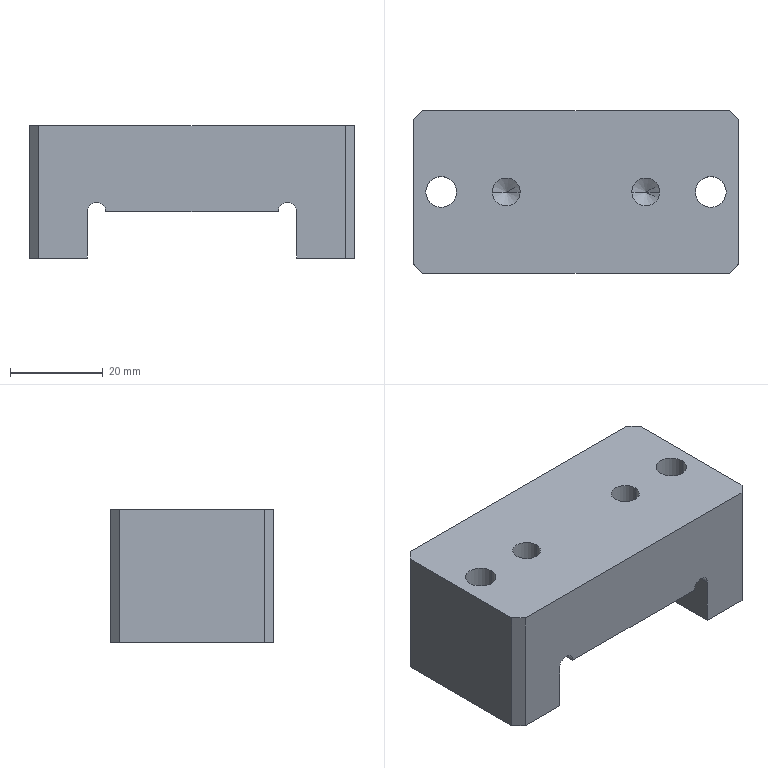Part | SolidWorks | features HoleWzd 3, Chamfer 1, Extrusion 1, ICE 1 | 1 solid | 52 faces | box 70 x 35 x 28.4 mm | volume 48866 mm3 | cylinder 24 | plane 16 | cone 12 | commonest cylinder face diameters 3.3 x8 4 x4 6 x4 6.6 x4 11 x4
STEP:
#1=CARTESIAN_POINT('',(30.65,12.5,-9.9));
#2=VERTEX_POINT('',#1);
#3=CARTESIAN_POINT('',(27.35,12.5,-9.9));
#4=VERTEX_POINT('',#3);
#5=CARTESIAN_POINT('',(29.,12.5,-9.9));
#6=DIRECTION('',(0.,0.,-1.));
#7=DIRECTION('',(-1.,0.,0.));
#8=AXIS2_PLACEMENT_3D('',#5,#6,#7);
#9=CIRCLE('',#8,1.65);
#10=EDGE_CURVE('',#2,#4,#9,.T.);
#11=ORIENTED_EDGE('',*,*,#10,.F.);
#12=CARTESIAN_POINT('',(30.65,12.5,-28.4));
#13=VERTEX_POINT('',#12);
#14=CARTESIAN_POINT('',(30.65,12.5,-28.4));
#15=DIRECTION('',(0.,0.,-1.));
#16=VECTOR('',#15,1000.);
#17=LINE('',#14,#16);
#18=EDGE_CURVE('',#2,#13,#17,.T.);
#19=ORIENTED_EDGE('',*,*,#18,.T.);
#20=CARTESIAN_POINT('',(27.35,12.5,-28.4));
#21=VERTEX_POINT('',#20);
#22=CARTESIAN_POINT('',(29.,12.5,-28.4));
#23=DIRECTION('',(0.,0.,-1.));
#24=DIRECTION('',(-1.,0.,0.));
#25=AXIS2_PLACEMENT_3D('',#22,#23,#24);
#26=CIRCLE('',#25,1.65);
#27=EDGE_CURVE('',#13,#21,#26,.T.);
#28=ORIENTED_EDGE('',*,*,#27,.T.);
#29=CARTESIAN_POINT('',(27.35,12.5,-28.4));
#30=DIRECTION('',(0.,0.,-1.));
#31=VECTOR('',#30,1000.);
#32=LINE('',#29,#31);
#33=EDGE_CURVE('',#4,#21,#32,.T.);
#34=ORIENTED_EDGE('',*,*,#33,.F.);
#35=EDGE_LOOP('',(#11,#19,#28,#34));
#36=FACE_OUTER_BOUND('',#35,.T.);
#37=CARTESIAN_POINT('',(29.,12.5,-28.4));
#38=DIRECTION('',(0.,0.,-1.));
#39=DIRECTION('',(-1.,0.,0.));
#40=AXIS2_PLACEMENT_3D('',#37,#38,#39);
#41=CYLINDRICAL_SURFACE('',#40,1.65);
#42=ADVANCED_FACE('',(#36),#41,.F.);
#43=CARTESIAN_POINT('',(29.,12.5,-8.909));
#44=VERTEX_POINT('',#43);
#45=CARTESIAN_POINT('',(27.35,12.5,-9.9));
#46=DIRECTION('',(-0.8572,0.,-0.515));
#47=VECTOR('',#46,1000.);
#48=LINE('',#45,#47);
#49=EDGE_CURVE('',#44,#4,#48,.T.);
#50=ORIENTED_EDGE('',*,*,#49,.F.);
#51=CARTESIAN_POINT('',(30.65,12.5,-9.9));
#52=DIRECTION('',(0.8572,0.,-0.515));
#53=VECTOR('',#52,1000.);
#54=LINE('',#51,#53);
#55=EDGE_CURVE('',#44,#2,#54,.T.);
#56=ORIENTED_EDGE('',*,*,#55,.T.);
#57=ORIENTED_EDGE('',*,*,#10,.T.);
#58=EDGE_LOOP('',(#50,#56,#57));
#59=FACE_OUTER_BOUND('',#58,.T.);
#60=CARTESIAN_POINT('',(29.,12.5,-9.9));
#61=DIRECTION('',(0.,0.,-1.));
#62=DIRECTION('',(-1.,0.,0.));
#63=AXIS2_PLACEMENT_3D('',#60,#61,#62);
#64=CONICAL_SURFACE('',#63,1.65,1.03);
#65=ADVANCED_FACE('',(#59),#64,.F.);
#66=CARTESIAN_POINT('',(30.65,-12.5,-9.9));
#67=VERTEX_POINT('',#66);
#68=CARTESIAN_POINT('',(27.35,-12.5,-9.9));
#69=VERTEX_POINT('',#68);
#70=CARTESIAN_POINT('',(29.,-12.5,-9.9));
#71=DIRECTION('',(0.,0.,-1.));
#72=DIRECTION('',(-1.,0.,0.));
#73=AXIS2_PLACEMENT_3D('',#70,#71,#72);
#74=CIRCLE('',#73,1.65);
#75=EDGE_CURVE('',#67,#69,#74,.T.);
#76=ORIENTED_EDGE('',*,*,#75,.F.);
#77=CARTESIAN_POINT('',(30.65,-12.5,-28.4));
#78=VERTEX_POINT('',#77);
#79=CARTESIAN_POINT('',(30.65,-12.5,-28.4));
#80=DIRECTION('',(0.,0.,-1.));
#81=VECTOR('',#80,1000.);
#82=LINE('',#79,#81);
#83=EDGE_CURVE('',#67,#78,#82,.T.);
#84=ORIENTED_EDGE('',*,*,#83,.T.);
#85=CARTESIAN_POINT('',(27.35,-12.5,-28.4));
#86=VERTEX_POINT('',#85);
#87=CARTESIAN_POINT('',(29.,-12.5,-28.4));
#88=DIRECTION('',(0.,0.,-1.));
#89=DIRECTION('',(-1.,0.,0.));
#90=AXIS2_PLACEMENT_3D('',#87,#88,#89);
#91=CIRCLE('',#90,1.65);
#92=EDGE_CURVE('',#78,#86,#91,.T.);
#93=ORIENTED_EDGE('',*,*,#92,.T.);
#94=CARTESIAN_POINT('',(27.35,-12.5,-28.4));
#95=DIRECTION('',(0.,0.,-1.));
#96=VECTOR('',#95,1000.);
#97=LINE('',#94,#96);
#98=EDGE_CURVE('',#69,#86,#97,.T.);
#99=ORIENTED_EDGE('',*,*,#98,.F.);
#100=EDGE_LOOP('',(#76,#84,#93,#99));
#101=FACE_OUTER_BOUND('',#100,.T.);
#102=CARTESIAN_POINT('',(29.,-12.5,-28.4));
#103=DIRECTION('',(0.,0.,-1.));
#104=DIRECTION('',(-1.,0.,0.));
#105=AXIS2_PLACEMENT_3D('',#102,#103,#104);
#106=CYLINDRICAL_SURFACE('',#105,1.65);
#107=ADVANCED_FACE('',(#101),#106,.F.);
#108=CARTESIAN_POINT('',(29.,-12.5,-8.909));
#109=VERTEX_POINT('',#108);
#110=CARTESIAN_POINT('',(27.35,-12.5,-9.9));
#111=DIRECTION('',(-0.8572,0.,-0.515));
#112=VECTOR('',#111,1000.);
#113=LINE('',#110,#112);
#114=EDGE_CURVE('',#109,#69,#113,.T.);
#115=ORIENTED_EDGE('',*,*,#114,.F.);
#116=CARTESIAN_POINT('',(30.65,-12.5,-9.9));
#117=DIRECTION('',(0.8572,0.,-0.515));
#118=VECTOR('',#117,1000.);
#119=LINE('',#116,#118);
#120=EDGE_CURVE('',#109,#67,#119,.T.);
#121=ORIENTED_EDGE('',*,*,#120,.T.);
#122=ORIENTED_EDGE('',*,*,#75,.T.);
#123=EDGE_LOOP('',(#115,#121,#122));
#124=FACE_OUTER_BOUND('',#123,.T.);
#125=CARTESIAN_POINT('',(29.,-12.5,-9.9));
#126=DIRECTION('',(0.,0.,-1.));
#127=DIRECTION('',(-1.,0.,0.));
#128=AXIS2_PLACEMENT_3D('',#125,#126,#127);
#129=CONICAL_SURFACE('',#128,1.65,1.03);
#130=ADVANCED_FACE('',(#124),#129,.F.);
#131=CARTESIAN_POINT('',(-27.35,12.5,-9.9));
#132=VERTEX_POINT('',#131);
#133=CARTESIAN_POINT('',(-30.65,12.5,-9.9));
#134=VERTEX_POINT('',#133);
#135=CARTESIAN_POINT('',(-29.,12.5,-9.9));
#136=DIRECTION('',(0.,0.,-1.));
#137=DIRECTION('',(-1.,0.,0.));
#138=AXIS2_PLACEMENT_3D('',#135,#136,#137);
#139=CIRCLE('',#138,1.65);
#140=EDGE_CURVE('',#132,#134,#139,.T.);
#141=ORIENTED_EDGE('',*,*,#140,.F.);
#142=CARTESIAN_POINT('',(-27.35,12.5,-28.4));
#143=VERTEX_POINT('',#142);
#144=CARTESIAN_POINT('',(-27.35,12.5,-28.4));
#145=DIRECTION('',(0.,0.,-1.));
#146=VECTOR('',#145,1000.);
#147=LINE('',#144,#146);
#148=EDGE_CURVE('',#132,#143,#147,.T.);
#149=ORIENTED_EDGE('',*,*,#148,.T.);
#150=CARTESIAN_POINT('',(-30.65,12.5,-28.4));
#151=VERTEX_POINT('',#150);
#152=CARTESIAN_POINT('',(-29.,12.5,-28.4));
#153=DIRECTION('',(0.,0.,-1.));
#154=DIRECTION('',(-1.,0.,0.));
#155=AXIS2_PLACEMENT_3D('',#152,#153,#154);
#156=CIRCLE('',#155,1.65);
#157=EDGE_CURVE('',#143,#151,#156,.T.);
#158=ORIENTED_EDGE('',*,*,#157,.T.);
#159=CARTESIAN_POINT('',(-30.65,12.5,-28.4));
#160=DIRECTION('',(0.,0.,-1.));
#161=VECTOR('',#160,1000.);
#162=LINE('',#159,#161);
#163=EDGE_CURVE('',#134,#151,#162,.T.);
#164=ORIENTED_EDGE('',*,*,#163,.F.);
#165=EDGE_LOOP('',(#141,#149,#158,#164));
#166=FACE_OUTER_BOUND('',#165,.T.);
#167=CARTESIAN_POINT('',(-29.,12.5,-28.4));
#168=DIRECTION('',(0.,0.,-1.));
#169=DIRECTION('',(-1.,0.,0.));
#170=AXIS2_PLACEMENT_3D('',#167,#168,#169);
#171=CYLINDRICAL_SURFACE('',#170,1.65);
#172=ADVANCED_FACE('',(#166),#171,.F.);
#173=CARTESIAN_POINT('',(-29.,12.5,-8.909));
#174=VERTEX_POINT('',#173);
#175=CARTESIAN_POINT('',(-30.65,12.5,-9.9));
#176=DIRECTION('',(-0.8572,0.,-0.515));
#177=VECTOR('',#176,1000.);
#178=LINE('',#175,#177);
#179=EDGE_CURVE('',#174,#134,#178,.T.);
#180=ORIENTED_EDGE('',*,*,#179,.F.);
#181=CARTESIAN_POINT('',(-27.35,12.5,-9.9));
#182=DIRECTION('',(0.8572,0.,-0.515));
#183=VECTOR('',#182,1000.);
#184=LINE('',#181,#183);
#185=EDGE_CURVE('',#174,#132,#184,.T.);
#186=ORIENTED_EDGE('',*,*,#185,.T.);
#187=ORIENTED_EDGE('',*,*,#140,.T.);
#188=EDGE_LOOP('',(#180,#186,#187));
#189=FACE_OUTER_BOUND('',#188,.T.);
#190=CARTESIAN_POINT('',(-29.,12.5,-9.9));
#191=DIRECTION('',(0.,0.,-1.));
#192=DIRECTION('',(-1.,0.,0.));
#193=AXIS2_PLACEMENT_3D('',#190,#191,#192);
#194=CONICAL_SURFACE('',#193,1.65,1.03);
#195=ADVANCED_FACE('',(#189),#194,.F.);
#196=CARTESIAN_POINT('',(-27.35,-12.5,-9.9));
#197=VERTEX_POINT('',#196);
#198=CARTESIAN_POINT('',(-30.65,-12.5,-9.9));
#199=VERTEX_POINT('',#198);
#200=CARTESIAN_POINT('',(-29.,-12.5,-9.9));
#201=DIRECTION('',(0.,0.,-1.));
#202=DIRECTION('',(-1.,0.,0.));
#203=AXIS2_PLACEMENT_3D('',#200,#201,#202);
#204=CIRCLE('',#203,1.65);
#205=EDGE_CURVE('',#197,#199,#204,.T.);
#206=ORIENTED_EDGE('',*,*,#205,.F.);
#207=CARTESIAN_POINT('',(-27.35,-12.5,-28.4));
#208=VERTEX_POINT('',#207);
#209=CARTESIAN_POINT('',(-27.35,-12.5,-28.4));
#210=DIRECTION('',(0.,0.,-1.));
#211=VECTOR('',#210,1000.);
#212=LINE('',#209,#211);
#213=EDGE_CURVE('',#197,#208,#212,.T.);
#214=ORIENTED_EDGE('',*,*,#213,.T.);
#215=CARTESIAN_POINT('',(-30.65,-12.5,-28.4));
#216=VERTEX_POINT('',#215);
#217=CARTESIAN_POINT('',(-29.,-12.5,-28.4));
#218=DIRECTION('',(0.,0.,-1.));
#219=DIRECTION('',(-1.,0.,0.));
#220=AXIS2_PLACEMENT_3D('',#217,#218,#219);
#221=CIRCLE('',#220,1.65);
#222=EDGE_CURVE('',#208,#216,#221,.T.);
#223=ORIENTED_EDGE('',*,*,#222,.T.);
#224=CARTESIAN_POINT('',(-30.65,-12.5,-28.4));
#225=DIRECTION('',(0.,0.,-1.));
#226=VECTOR('',#225,1000.);
#227=LINE('',#224,#226);
#228=EDGE_CURVE('',#199,#216,#227,.T.);
#229=ORIENTED_EDGE('',*,*,#228,.F.);
#230=EDGE_LOOP('',(#206,#214,#223,#229));
#231=FACE_OUTER_BOUND('',#230,.T.);
#232=CARTESIAN_POINT('',(-29.,-12.5,-28.4));
#233=DIRECTION('',(0.,0.,-1.));
#234=DIRECTION('',(-1.,0.,0.));
#235=AXIS2_PLACEMENT_3D('',#232,#233,#234);
#236=CYLINDRICAL_SURFACE('',#235,1.65);
#237=ADVANCED_FACE('',(#231),#236,.F.);
#238=CARTESIAN_POINT('',(-29.,-12.5,-8.909));
#239=VERTEX_POINT('',#238);
#240=CARTESIAN_POINT('',(-30.65,-12.5,-9.9));
#241=DIRECTION('',(-0.8572,0.,-0.515));
#242=VECTOR('',#241,1000.);
#243=LINE('',#240,#242);
#244=EDGE_CURVE('',#239,#199,#243,.T.);
#245=ORIENTED_EDGE('',*,*,#244,.F.);
#246=CARTESIAN_POINT('',(-27.35,-12.5,-9.9));
#247=DIRECTION('',(0.8572,0.,-0.515));
#248=VECTOR('',#247,1000.);
#249=LINE('',#246,#248);
#250=EDGE_CURVE('',#239,#197,#249,.T.);
#251=ORIENTED_EDGE('',*,*,#250,.T.);
#252=ORIENTED_EDGE('',*,*,#205,.T.);
#253=EDGE_LOOP('',(#245,#251,#252));
#254=FACE_OUTER_BOUND('',#253,.T.);
#255=CARTESIAN_POINT('',(-29.,-12.5,-9.9));
#256=DIRECTION('',(0.,0.,-1.));
#257=DIRECTION('',(-1.,0.,0.));
#258=AXIS2_PLACEMENT_3D('',#255,#256,#257);
#259=CONICAL_SURFACE('',#258,1.65,1.03);
#260=ADVANCED_FACE('',(#254),#259,.F.);
#261=CARTESIAN_POINT('',(34.5,0.,-21.6));
#262=VERTEX_POINT('',#261);
#263=CARTESIAN_POINT('',(23.5,0.,-21.6));
#264=VERTEX_POINT('',#263);
#265=CARTESIAN_POINT('',(29.,0.,-21.6));
#266=DIRECTION('',(0.,0.,-1.));
#267=DIRECTION('',(-1.,0.,0.));
#268=AXIS2_PLACEMENT_3D('',#265,#266,#267);
#269=CIRCLE('',#268,5.5);
#270=EDGE_CURVE('',#262,#264,#269,.T.);
#271=ORIENTED_EDGE('',*,*,#270,.F.);
#272=CARTESIAN_POINT('',(34.5,0.,-28.4));
#273=VERTEX_POINT('',#272);
#274=CARTESIAN_POINT('',(34.5,0.,-28.4));
#275=DIRECTION('',(0.,0.,-1.));
#276=VECTOR('',#275,1000.);
#277=LINE('',#274,#276);
#278=EDGE_CURVE('',#262,#273,#277,.T.);
#279=ORIENTED_EDGE('',*,*,#278,.T.);
#280=CARTESIAN_POINT('',(23.5,0.,-28.4));
#281=VERTEX_POINT('',#280);
#282=CARTESIAN_POINT('',(29.,0.,-28.4));
#283=DIRECTION('',(0.,0.,-1.));
#284=DIRECTION('',(-1.,0.,0.));
#285=AXIS2_PLACEMENT_3D('',#282,#283,#284);
#286=CIRCLE('',#285,5.5);
#287=EDGE_CURVE('',#273,#281,#286,.T.);
#288=ORIENTED_EDGE('',*,*,#287,.T.);
#289=CARTESIAN_POINT('',(23.5,0.,-28.4));
#290=DIRECTION('',(0.,0.,-1.));
#291=VECTOR('',#290,1000.);
#292=LINE('',#289,#291);
#293=EDGE_CURVE('',#264,#281,#292,.T.);
#294=ORIENTED_EDGE('',*,*,#293,.F.);
#295=EDGE_LOOP('',(#271,#279,#288,#294));
#296=FACE_OUTER_BOUND('',#295,.T.);
#297=CARTESIAN_POINT('',(29.,0.,-28.4));
#298=DIRECTION('',(0.,0.,-1.));
#299=DIRECTION('',(-1.,0.,0.));
#300=AXIS2_PLACEMENT_3D('',#297,#298,#299);
#301=CYLINDRICAL_SURFACE('',#300,5.5);
#302=ADVANCED_FACE('',(#296),#301,.F.);
#303=CARTESIAN_POINT('',(32.3,0.,0.));
#304=VERTEX_POINT('',#303);
#305=CARTESIAN_POINT('',(25.7,0.,0.));
#306=VERTEX_POINT('',#305);
#307=CARTESIAN_POINT('',(29.,0.,0.));
#308=DIRECTION('',(0.,0.,-1.));
#309=DIRECTION('',(-1.,0.,0.));
#310=AXIS2_PLACEMENT_3D('',#307,#308,#309);
#311=CIRCLE('',#310,3.3);
#312=EDGE_CURVE('',#304,#306,#311,.T.);
#313=ORIENTED_EDGE('',*,*,#312,.F.);
#314=CARTESIAN_POINT('',(32.3,0.,-21.6));
#315=VERTEX_POINT('',#314);
#316=CARTESIAN_POINT('',(32.3,0.,-28.4));
#317=DIRECTION('',(0.,0.,-1.));
#318=VECTOR('',#317,1000.);
#319=LINE('',#316,#318);
#320=EDGE_CURVE('',#304,#315,#319,.T.);
#321=ORIENTED_EDGE('',*,*,#320,.T.);
#322=CARTESIAN_POINT('',(25.7,0.,-21.6));
#323=VERTEX_POINT('',#322);
#324=CARTESIAN_POINT('',(29.,0.,-21.6));
#325=DIRECTION('',(0.,0.,-1.));
#326=DIRECTION('',(-1.,0.,0.));
#327=AXIS2_PLACEMENT_3D('',#324,#325,#326);
#328=CIRCLE('',#327,3.3);
#329=EDGE_CURVE('',#315,#323,#328,.T.);
#330=ORIENTED_EDGE('',*,*,#329,.T.);
#331=CARTESIAN_POINT('',(25.7,0.,-28.4));
#332=DIRECTION('',(0.,0.,-1.));
#333=VECTOR('',#332,1000.);
#334=LINE('',#331,#333);
#335=EDGE_CURVE('',#306,#323,#334,.T.);
#336=ORIENTED_EDGE('',*,*,#335,.F.);
#337=EDGE_LOOP('',(#313,#321,#330,#336));
#338=FACE_OUTER_BOUND('',#337,.T.);
#339=CARTESIAN_POINT('',(29.,0.,-28.4));
#340=DIRECTION('',(0.,0.,-1.));
#341=DIRECTION('',(-1.,0.,0.));
#342=AXIS2_PLACEMENT_3D('',#339,#340,#341);
#343=CYLINDRICAL_SURFACE('',#342,3.3);
#344=ADVANCED_FACE('',(#338),#343,.F.);
#345=CARTESIAN_POINT('',(-23.5,0.,-21.6));
#346=VERTEX_POINT('',#345);
#347=CARTESIAN_POINT('',(-34.5,0.,-21.6));
#348=VERTEX_POINT('',#347);
#349=CARTESIAN_POINT('',(-29.,0.,-21.6));
#350=DIRECTION('',(0.,0.,-1.));
#351=DIRECTION('',(-1.,0.,0.));
#352=AXIS2_PLACEMENT_3D('',#349,#350,#351);
#353=CIRCLE('',#352,5.5);
#354=EDGE_CURVE('',#346,#348,#353,.T.);
#355=ORIENTED_EDGE('',*,*,#354,.F.);
#356=CARTESIAN_POINT('',(-23.5,0.,-28.4));
#357=VERTEX_POINT('',#356);
#358=CARTESIAN_POINT('',(-23.5,0.,-28.4));
#359=DIRECTION('',(0.,0.,-1.));
#360=VECTOR('',#359,1000.);
#361=LINE('',#358,#360);
#362=EDGE_CURVE('',#346,#357,#361,.T.);
#363=ORIENTED_EDGE('',*,*,#362,.T.);
#364=CARTESIAN_POINT('',(-34.5,0.,-28.4));
#365=VERTEX_POINT('',#364);
#366=CARTESIAN_POINT('',(-29.,0.,-28.4));
#367=DIRECTION('',(0.,0.,-1.));
#368=DIRECTION('',(-1.,0.,0.));
#369=AXIS2_PLACEMENT_3D('',#366,#367,#368);
#370=CIRCLE('',#369,5.5);
#371=EDGE_CURVE('',#357,#365,#370,.T.);
#372=ORIENTED_EDGE('',*,*,#371,.T.);
#373=CARTESIAN_POINT('',(-34.5,0.,-28.4));
#374=DIRECTION('',(0.,0.,-1.));
#375=VECTOR('',#374,1000.);
#376=LINE('',#373,#375);
#377=EDGE_CURVE('',#348,#365,#376,.T.);
#378=ORIENTED_EDGE('',*,*,#377,.F.);
#379=EDGE_LOOP('',(#355,#363,#372,#378));
#380=FACE_OUTER_BOUND('',#379,.T.);
#381=CARTESIAN_POINT('',(-29.,0.,-28.4));
#382=DIRECTION('',(0.,0.,-1.));
#383=DIRECTION('',(-1.,0.,0.));
#384=AXIS2_PLACEMENT_3D('',#381,#382,#383);
#385=CYLINDRICAL_SURFACE('',#384,5.5);
#386=ADVANCED_FACE('',(#380),#385,.F.);
#387=CARTESIAN_POINT('',(-25.7,0.,0.));
#388=VERTEX_POINT('',#387);
#389=CARTESIAN_POINT('',(-32.3,0.,0.));
#390=VERTEX_POINT('',#389);
#391=CARTESIAN_POINT('',(-29.,0.,0.));
#392=DIRECTION('',(0.,0.,-1.));
#393=DIRECTION('',(-1.,0.,0.));
#394=AXIS2_PLACEMENT_3D('',#391,#392,#393);
#395=CIRCLE('',#394,3.3);
#396=EDGE_CURVE('',#388,#390,#395,.T.);
#397=ORIENTED_EDGE('',*,*,#396,.F.);
#398=CARTESIAN_POINT('',(-25.7,0.,-21.6));
#399=VERTEX_POINT('',#398);
#400=CARTESIAN_POINT('',(-25.7,0.,-28.4));
#401=DIRECTION('',(0.,0.,-1.));
#402=VECTOR('',#401,1000.);
#403=LINE('',#400,#402);
#404=EDGE_CURVE('',#388,#399,#403,.T.);
#405=ORIENTED_EDGE('',*,*,#404,.T.);
#406=CARTESIAN_POINT('',(-32.3,0.,-21.6));
#407=VERTEX_POINT('',#406);
#408=CARTESIAN_POINT('',(-29.,0.,-21.6));
#409=DIRECTION('',(0.,0.,-1.));
#410=DIRECTION('',(-1.,0.,0.));
#411=AXIS2_PLACEMENT_3D('',#408,#409,#410);
#412=CIRCLE('',#411,3.3);
#413=EDGE_CURVE('',#399,#407,#412,.T.);
#414=ORIENTED_EDGE('',*,*,#413,.T.);
#415=CARTESIAN_POINT('',(-32.3,0.,-28.4));
#416=DIRECTION('',(0.,0.,-1.));
#417=VECTOR('',#416,1000.);
#418=LINE('',#415,#417);
#419=EDGE_CURVE('',#390,#407,#418,.T.);
#420=ORIENTED_EDGE('',*,*,#419,.F.);
#421=EDGE_LOOP('',(#397,#405,#414,#420));
#422=FACE_OUTER_BOUND('',#421,.T.);
#423=CARTESIAN_POINT('',(-29.,0.,-28.4));
#424=DIRECTION('',(0.,0.,-1.));
#425=DIRECTION('',(-1.,0.,0.));
#426=AXIS2_PLACEMENT_3D('',#423,#424,#425);
#427=CYLINDRICAL_SURFACE('',#426,3.3);
#428=ADVANCED_FACE('',(#422),#427,.F.);
#429=CARTESIAN_POINT('',(-18.,0.,-15.));
#430=VERTEX_POINT('',#429);
#431=CARTESIAN_POINT('',(-12.,0.,-15.));
#432=VERTEX_POINT('',#431);
#433=CARTESIAN_POINT('',(-15.,0.,-15.));
#434=DIRECTION('',(0.,0.,1.));
#435=DIRECTION('',(1.,0.,0.));
#436=AXIS2_PLACEMENT_3D('',#433,#434,#435);
#437=CIRCLE('',#436,3.);
#438=EDGE_CURVE('',#430,#432,#437,.T.);
#439=ORIENTED_EDGE('',*,*,#438,.F.);
#440=CARTESIAN_POINT('',(-18.,0.,0.));
#441=VERTEX_POINT('',#440);
#442=CARTESIAN_POINT('',(-18.,0.,0.));
#443=DIRECTION('',(0.,0.,1.));
#444=VECTOR('',#443,1000.);
#445=LINE('',#442,#444);
#446=EDGE_CURVE('',#430,#441,#445,.T.);
#447=ORIENTED_EDGE('',*,*,#446,.T.);
#448=CARTESIAN_POINT('',(-12.,0.,0.));
#449=VERTEX_POINT('',#448);
#450=CARTESIAN_POINT('',(-15.,0.,0.));
#451=DIRECTION('',(0.,0.,1.));
#452=DIRECTION('',(1.,0.,0.));
#453=AXIS2_PLACEMENT_3D('',#450,#451,#452);
#454=CIRCLE('',#453,3.);
#455=EDGE_CURVE('',#441,#449,#454,.T.);
#456=ORIENTED_EDGE('',*,*,#455,.T.);
#457=CARTESIAN_POINT('',(-12.,0.,0.));
#458=DIRECTION('',(0.,0.,1.));
#459=VECTOR('',#458,1000.);
#460=LINE('',#457,#459);
#461=EDGE_CURVE('',#432,#449,#460,.T.);
#462=ORIENTED_EDGE('',*,*,#461,.F.);
#463=EDGE_LOOP('',(#439,#447,#456,#462));
#464=FACE_OUTER_BOUND('',#463,.T.);
#465=CARTESIAN_POINT('',(-15.,0.,0.));
#466=DIRECTION('',(0.,0.,1.));
#467=DIRECTION('',(1.,0.,0.));
#468=AXIS2_PLACEMENT_3D('',#465,#466,#467);
#469=CYLINDRICAL_SURFACE('',#468,3.);
#470=ADVANCED_FACE('',(#464),#469,.F.);
#471=CARTESIAN_POINT('',(-15.,0.,-16.803));
#472=VERTEX_POINT('',#471);
#473=CARTESIAN_POINT('',(-12.,0.,-15.));
#474=DIRECTION('',(0.8572,0.,0.515));
#475=VECTOR('',#474,1000.);
#476=LINE('',#473,#475);
#477=EDGE_CURVE('',#472,#432,#476,.T.);
#478=ORIENTED_EDGE('',*,*,#477,.F.);
#479=CARTESIAN_POINT('',(-18.,0.,-15.));
#480=DIRECTION('',(-0.8572,0.,0.515));
#481=VECTOR('',#480,1000.);
#482=LINE('',#479,#481);
#483=EDGE_CURVE('',#472,#430,#482,.T.);
#484=ORIENTED_EDGE('',*,*,#483,.T.);
#485=ORIENTED_EDGE('',*,*,#438,.T.);
#486=EDGE_LOOP('',(#478,#484,#485));
#487=FACE_OUTER_BOUND('',#486,.T.);
#488=CARTESIAN_POINT('',(-15.,0.,-15.));
#489=DIRECTION('',(0.,0.,1.));
#490=DIRECTION('',(1.,0.,0.));
#491=AXIS2_PLACEMENT_3D('',#488,#489,#490);
#492=CONICAL_SURFACE('',#491,3.,1.03);
#493=ADVANCED_FACE('',(#487),#492,.F.);
#494=CARTESIAN_POINT('',(12.,0.,-15.));
#495=VERTEX_POINT('',#494);
#496=CARTESIAN_POINT('',(18.,0.,-15.));
#497=VERTEX_POINT('',#496);
#498=CARTESIAN_POINT('',(15.,0.,-15.));
#499=DIRECTION('',(0.,0.,1.));
#500=DIRECTION('',(1.,0.,0.));
#501=AXIS2_PLACEMENT_3D('',#498,#499,#500);
#502=CIRCLE('',#501,3.);
#503=EDGE_CURVE('',#495,#497,#502,.T.);
#504=ORIENTED_EDGE('',*,*,#503,.F.);
#505=CARTESIAN_POINT('',(12.,0.,0.));
#506=VERTEX_POINT('',#505);
#507=CARTESIAN_POINT('',(12.,0.,0.));
#508=DIRECTION('',(0.,0.,1.));
#509=VECTOR('',#508,1000.);
#510=LINE('',#507,#509);
#511=EDGE_CURVE('',#495,#506,#510,.T.);
#512=ORIENTED_EDGE('',*,*,#511,.T.);
#513=CARTESIAN_POINT('',(18.,0.,0.));
#514=VERTEX_POINT('',#513);
#515=CARTESIAN_POINT('',(15.,0.,0.));
#516=DIRECTION('',(0.,0.,1.));
#517=DIRECTION('',(1.,0.,0.));
#518=AXIS2_PLACEMENT_3D('',#515,#516,#517);
#519=CIRCLE('',#518,3.);
#520=EDGE_CURVE('',#506,#514,#519,.T.);
#521=ORIENTED_EDGE('',*,*,#520,.T.);
#522=CARTESIAN_POINT('',(18.,0.,0.));
#523=DIRECTION('',(0.,0.,1.));
#524=VECTOR('',#523,1000.);
#525=LINE('',#522,#524);
#526=EDGE_CURVE('',#497,#514,#525,.T.);
#527=ORIENTED_EDGE('',*,*,#526,.F.);
#528=EDGE_LOOP('',(#504,#512,#521,#527));
#529=FACE_OUTER_BOUND('',#528,.T.);
#530=CARTESIAN_POINT('',(15.,0.,0.));
#531=DIRECTION('',(0.,0.,1.));
#532=DIRECTION('',(1.,0.,0.));
#533=AXIS2_PLACEMENT_3D('',#530,#531,#532);
#534=CYLINDRICAL_SURFACE('',#533,3.);
#535=ADVANCED_FACE('',(#529),#534,.F.);
#536=CARTESIAN_POINT('',(15.,0.,-16.803));
#537=VERTEX_POINT('',#536);
#538=CARTESIAN_POINT('',(18.,0.,-15.));
#539=DIRECTION('',(0.8572,0.,0.515));
#540=VECTOR('',#539,1000.);
#541=LINE('',#538,#540);
#542=EDGE_CURVE('',#537,#497,#541,.T.);
#543=ORIENTED_EDGE('',*,*,#542,.F.);
#544=CARTESIAN_POINT('',(12.,0.,-15.));
#545=DIRECTION('',(-0.8572,0.,0.515));
#546=VECTOR('',#545,1000.);
#547=LINE('',#544,#546);
#548=EDGE_CURVE('',#537,#495,#547,.T.);
#549=ORIENTED_EDGE('',*,*,#548,.T.);
#550=ORIENTED_EDGE('',*,*,#503,.T.);
#551=EDGE_LOOP('',(#543,#549,#550));
#552=FACE_OUTER_BOUND('',#551,.T.);
#553=CARTESIAN_POINT('',(15.,0.,-15.));
#554=DIRECTION('',(0.,0.,1.));
#555=DIRECTION('',(1.,0.,0.));
#556=AXIS2_PLACEMENT_3D('',#553,#554,#555);
#557=CONICAL_SURFACE('',#556,3.,1.03);
#558=ADVANCED_FACE('',(#552),#557,.F.);
#559=CARTESIAN_POINT('',(-18.5,-17.5,-18.4));
#560=VERTEX_POINT('',#559);
#561=CARTESIAN_POINT('',(-20.5,-17.5,-16.4));
#562=VERTEX_POINT('',#561);
#563=CARTESIAN_POINT('',(-20.5,-17.5,-18.4));
#564=DIRECTION('',(0.,-1.,0.));
#565=DIRECTION('',(0.,0.,1.));
#566=AXIS2_PLACEMENT_3D('',#563,#564,#565);
#567=CIRCLE('',#566,2.);
#568=EDGE_CURVE('',#560,#562,#567,.T.);
#569=ORIENTED_EDGE('',*,*,#568,.T.);
#570=CARTESIAN_POINT('',(-20.5,17.5,-16.4));
#571=VERTEX_POINT('',#570);
#572=CARTESIAN_POINT('',(-20.5,-17.501,-16.4));
#573=DIRECTION('',(0.,1.,0.));
#574=VECTOR('',#573,1000.);
#575=LINE('',#572,#574);
#576=EDGE_CURVE('',#562,#571,#575,.T.);
#577=ORIENTED_EDGE('',*,*,#576,.T.);
#578=CARTESIAN_POINT('',(-18.5,17.5,-18.4));
#579=VERTEX_POINT('',#578);
#580=CARTESIAN_POINT('',(-20.5,17.5,-18.4));
#581=DIRECTION('',(0.,1.,0.));
#582=DIRECTION('',(0.,0.,1.));
#583=AXIS2_PLACEMENT_3D('',#580,#581,#582);
#584=CIRCLE('',#583,2.);
#585=EDGE_CURVE('',#571,#579,#584,.T.);
#586=ORIENTED_EDGE('',*,*,#585,.T.);
#587=CARTESIAN_POINT('',(-18.5,-17.501,-18.4));
#588=DIRECTION('',(0.,-1.,0.));
#589=VECTOR('',#588,1000.);
#590=LINE('',#587,#589);
#591=EDGE_CURVE('',#579,#560,#590,.T.);
#592=ORIENTED_EDGE('',*,*,#591,.T.);
#593=EDGE_LOOP('',(#569,#577,#586,#592));
#594=FACE_OUTER_BOUND('',#593,.T.);
#595=CARTESIAN_POINT('',(-20.5,-17.501,-18.4));
#596=DIRECTION('',(0.,1.,0.));
#597=DIRECTION('',(0.,0.,1.));
#598=AXIS2_PLACEMENT_3D('',#595,#596,#597);
#599=CYLINDRICAL_SURFACE('',#598,2.);
#600=ADVANCED_FACE('',(#594),#599,.F.);
#601=CARTESIAN_POINT('',(22.5,-17.5,-18.4));
#602=VERTEX_POINT('',#601);
#603=CARTESIAN_POINT('',(20.5,-17.5,-16.4));
#604=VERTEX_POINT('',#603);
#605=CARTESIAN_POINT('',(20.5,-17.5,-18.4));
#606=DIRECTION('',(0.,-1.,0.));
#607=DIRECTION('',(0.,0.,1.));
#608=AXIS2_PLACEMENT_3D('',#605,#606,#607);
#609=CIRCLE('',#608,2.);
#610=EDGE_CURVE('',#602,#604,#609,.T.);
#611=ORIENTED_EDGE('',*,*,#610,.T.);
#612=CARTESIAN_POINT('',(20.5,17.5,-16.4));
#613=VERTEX_POINT('',#612);
#614=CARTESIAN_POINT('',(20.5,-17.501,-16.4));
#615=DIRECTION('',(0.,1.,0.));
#616=VECTOR('',#615,1000.);
#617=LINE('',#614,#616);
#618=EDGE_CURVE('',#604,#613,#617,.T.);
#619=ORIENTED_EDGE('',*,*,#618,.T.);
#620=CARTESIAN_POINT('',(22.5,17.5,-18.4));
#621=VERTEX_POINT('',#620);
#622=CARTESIAN_POINT('',(20.5,17.5,-18.4));
#623=DIRECTION('',(0.,1.,0.));
#624=DIRECTION('',(0.,0.,1.));
#625=AXIS2_PLACEMENT_3D('',#622,#623,#624);
#626=CIRCLE('',#625,2.);
#627=EDGE_CURVE('',#613,#621,#626,.T.);
#628=ORIENTED_EDGE('',*,*,#627,.T.);
#629=CARTESIAN_POINT('',(22.5,17.5,-18.4));
#630=DIRECTION('',(0.,-1.,0.));
#631=VECTOR('',#630,1000.);
#632=LINE('',#629,#631);
#633=EDGE_CURVE('',#621,#602,#632,.T.);
#634=ORIENTED_EDGE('',*,*,#633,.T.);
#635=EDGE_LOOP('',(#611,#619,#628,#634));
#636=FACE_OUTER_BOUND('',#635,.T.);
#637=CARTESIAN_POINT('',(20.5,-17.501,-18.4));
#638=DIRECTION('',(0.,1.,0.));
#639=DIRECTION('',(0.,0.,1.));
#640=AXIS2_PLACEMENT_3D('',#637,#638,#639);
#641=CYLINDRICAL_SURFACE('',#640,2.);
#642=ADVANCED_FACE('',(#636),#641,.F.);
#643=CARTESIAN_POINT('',(29.,12.5,-28.4));
#644=DIRECTION('',(0.,0.,-1.));
#645=DIRECTION('',(-1.,0.,0.));
#646=AXIS2_PLACEMENT_3D('',#643,#644,#645);
#647=CIRCLE('',#646,1.65);
#648=EDGE_CURVE('',#21,#13,#647,.T.);
#649=ORIENTED_EDGE('',*,*,#648,.F.);
#650=ORIENTED_EDGE('',*,*,#27,.F.);
#651=EDGE_LOOP('',(#649,#650));
#652=FACE_BOUND('',#651,.T.);
#653=CARTESIAN_POINT('',(29.,-12.5,-28.4));
#654=DIRECTION('',(0.,0.,-1.));
#655=DIRECTION('',(-1.,0.,0.));
#656=AXIS2_PLACEMENT_3D('',#653,#654,#655);
#657=CIRCLE('',#656,1.65);
#658=EDGE_CURVE('',#86,#78,#657,.T.);
#659=ORIENTED_EDGE('',*,*,#658,.F.);
#660=ORIENTED_EDGE('',*,*,#92,.F.);
#661=EDGE_LOOP('',(#659,#660));
#662=FACE_BOUND('',#661,.T.);
#663=CARTESIAN_POINT('',(35.,15.5,-28.4));
#664=VERTEX_POINT('',#663);
#665=CARTESIAN_POINT('',(35.,-15.5,-28.4));
#666=VERTEX_POINT('',#665);
#667=CARTESIAN_POINT('',(35.,17.5,-28.4));
#668=DIRECTION('',(0.,-1.,0.));
#669=VECTOR('',#668,1000.);
#670=LINE('',#667,#669);
#671=EDGE_CURVE('',#664,#666,#670,.T.);
#672=ORIENTED_EDGE('',*,*,#671,.T.);
#673=CARTESIAN_POINT('',(33.,-17.5,-28.4));
#674=VERTEX_POINT('',#673);
#675=CARTESIAN_POINT('',(35.,-15.5,-28.4));
#676=DIRECTION('',(-0.7071,-0.7071,0.));
#677=VECTOR('',#676,1000.);
#678=LINE('',#675,#677);
#679=EDGE_CURVE('',#666,#674,#678,.T.);
#680=ORIENTED_EDGE('',*,*,#679,.T.);
#681=CARTESIAN_POINT('',(22.5,-17.5,-28.4));
#682=VERTEX_POINT('',#681);
#683=CARTESIAN_POINT('',(35.,-17.5,-28.4));
#684=DIRECTION('',(-1.,0.,0.));
#685=VECTOR('',#684,1000.);
#686=LINE('',#683,#685);
#687=EDGE_CURVE('',#674,#682,#686,.T.);
#688=ORIENTED_EDGE('',*,*,#687,.T.);
#689=CARTESIAN_POINT('',(22.5,17.5,-28.4));
#690=VERTEX_POINT('',#689);
#691=CARTESIAN_POINT('',(22.5,17.5,-28.4));
#692=DIRECTION('',(0.,-1.,0.));
#693=VECTOR('',#692,1000.);
#694=LINE('',#691,#693);
#695=EDGE_CURVE('',#690,#682,#694,.T.);
#696=ORIENTED_EDGE('',*,*,#695,.F.);
#697=CARTESIAN_POINT('',(33.,17.5,-28.4));
#698=VERTEX_POINT('',#697);
#699=CARTESIAN_POINT('',(35.,17.5,-28.4));
#700=DIRECTION('',(-1.,0.,0.));
#701=VECTOR('',#700,1000.);
#702=LINE('',#699,#701);
#703=EDGE_CURVE('',#698,#690,#702,.T.);
#704=ORIENTED_EDGE('',*,*,#703,.F.);
#705=CARTESIAN_POINT('',(33.,17.5,-28.4));
#706=DIRECTION('',(0.7071,-0.7071,0.));
#707=VECTOR('',#706,1000.);
#708=LINE('',#705,#707);
#709=EDGE_CURVE('',#698,#664,#708,.T.);
#710=ORIENTED_EDGE('',*,*,#709,.T.);
#711=EDGE_LOOP('',(#672,#680,#688,#696,#704,#710));
#712=FACE_OUTER_BOUND('',#711,.T.);
#713=CARTESIAN_POINT('',(29.,0.,-28.4));
#714=DIRECTION('',(0.,0.,-1.));
#715=DIRECTION('',(-1.,0.,0.));
#716=AXIS2_PLACEMENT_3D('',#713,#714,#715);
#717=CIRCLE('',#716,5.5);
#718=EDGE_CURVE('',#281,#273,#717,.T.);
#719=ORIENTED_EDGE('',*,*,#718,.F.);
#720=ORIENTED_EDGE('',*,*,#287,.F.);
#721=EDGE_LOOP('',(#719,#720));
#722=FACE_BOUND('',#721,.T.);
#723=CARTESIAN_POINT('',(35.,17.5,-28.4));
#724=DIRECTION('',(0.,0.,1.));
#725=DIRECTION('',(1.,0.,0.));
#726=AXIS2_PLACEMENT_3D('',#723,#724,#725);
#727=PLANE('',#726);
#728=ADVANCED_FACE('',(#652,#662,#712,#722),#727,.F.);
#729=CARTESIAN_POINT('',(-29.,12.5,-28.4));
#730=DIRECTION('',(0.,0.,-1.));
#731=DIRECTION('',(-1.,0.,0.));
#732=AXIS2_PLACEMENT_3D('',#729,#730,#731);
#733=CIRCLE('',#732,1.65);
#734=EDGE_CURVE('',#151,#143,#733,.T.);
#735=ORIENTED_EDGE('',*,*,#734,.F.);
#736=ORIENTED_EDGE('',*,*,#157,.F.);
#737=EDGE_LOOP('',(#735,#736));
#738=FACE_BOUND('',#737,.T.);
#739=CARTESIAN_POINT('',(-29.,-12.5,-28.4));
#740=DIRECTION('',(0.,0.,-1.));
#741=DIRECTION('',(-1.,0.,0.));
#742=AXIS2_PLACEMENT_3D('',#739,#740,#741);
#743=CIRCLE('',#742,1.65);
#744=EDGE_CURVE('',#216,#208,#743,.T.);
#745=ORIENTED_EDGE('',*,*,#744,.F.);
#746=ORIENTED_EDGE('',*,*,#222,.F.);
#747=EDGE_LOOP('',(#745,#746));
#748=FACE_BOUND('',#747,.T.);
#749=CARTESIAN_POINT('',(-22.5,-17.5,-28.4));
#750=VERTEX_POINT('',#749);
#751=CARTESIAN_POINT('',(-33.,-17.5,-28.4));
#752=VERTEX_POINT('',#751);
#753=CARTESIAN_POINT('',(-22.5,-17.5,-28.4));
#754=DIRECTION('',(-1.,0.,0.));
#755=VECTOR('',#754,1000.);
#756=LINE('',#753,#755);
#757=EDGE_CURVE('',#750,#752,#756,.T.);
#758=ORIENTED_EDGE('',*,*,#757,.T.);
#759=CARTESIAN_POINT('',(-35.,-15.5,-28.4));
#760=VERTEX_POINT('',#759);
#761=CARTESIAN_POINT('',(-35.,-15.5,-28.4));
#762=DIRECTION('',(-0.7071,0.7071,0.));
#763=VECTOR('',#762,1000.);
#764=LINE('',#761,#763);
#765=EDGE_CURVE('',#752,#760,#764,.T.);
#766=ORIENTED_EDGE('',*,*,#765,.T.);
#767=CARTESIAN_POINT('',(-35.,15.5,-28.4));
#768=VERTEX_POINT('',#767);
#769=CARTESIAN_POINT('',(-35.,17.5,-28.4));
#770=DIRECTION('',(0.,-1.,0.));
#771=VECTOR('',#770,1000.);
#772=LINE('',#769,#771);
#773=EDGE_CURVE('',#768,#760,#772,.T.);
#774=ORIENTED_EDGE('',*,*,#773,.F.);
#775=CARTESIAN_POINT('',(-33.,17.5,-28.4));
#776=VERTEX_POINT('',#775);
#777=CARTESIAN_POINT('',(-33.,17.5,-28.4));
#778=DIRECTION('',(0.7071,0.7071,0.));
#779=VECTOR('',#778,1000.);
#780=LINE('',#777,#779);
#781=EDGE_CURVE('',#768,#776,#780,.T.);
#782=ORIENTED_EDGE('',*,*,#781,.T.);
#783=CARTESIAN_POINT('',(-22.5,17.5,-28.4));
#784=VERTEX_POINT('',#783);
#785=CARTESIAN_POINT('',(-22.5,17.5,-28.4));
#786=DIRECTION('',(-1.,0.,0.));
#787=VECTOR('',#786,1000.);
#788=LINE('',#785,#787);
#789=EDGE_CURVE('',#784,#776,#788,.T.);
#790=ORIENTED_EDGE('',*,*,#789,.F.);
#791=CARTESIAN_POINT('',(-22.5,17.5,-28.4));
#792=DIRECTION('',(0.,-1.,0.));
#793=VECTOR('',#792,1000.);
#794=LINE('',#791,#793);
#795=EDGE_CURVE('',#784,#750,#794,.T.);
#796=ORIENTED_EDGE('',*,*,#795,.T.);
#797=EDGE_LOOP('',(#758,#766,#774,#782,#790,#796));
#798=FACE_OUTER_BOUND('',#797,.T.);
#799=CARTESIAN_POINT('',(-29.,0.,-28.4));
#800=DIRECTION('',(0.,0.,-1.));
#801=DIRECTION('',(-1.,0.,0.));
#802=AXIS2_PLACEMENT_3D('',#799,#800,#801);
#803=CIRCLE('',#802,5.5);
#804=EDGE_CURVE('',#365,#357,#803,.T.);
#805=ORIENTED_EDGE('',*,*,#804,.F.);
#806=ORIENTED_EDGE('',*,*,#371,.F.);
#807=EDGE_LOOP('',(#805,#806));
#808=FACE_BOUND('',#807,.T.);
#809=CARTESIAN_POINT('',(-22.5,17.5,-28.4));
#810=DIRECTION('',(0.,0.,1.));
#811=DIRECTION('',(1.,0.,0.));
#812=AXIS2_PLACEMENT_3D('',#809,#810,#811);
#813=PLANE('',#812);
#814=ADVANCED_FACE('',(#738,#748,#798,#808),#813,.F.);
#815=ORIENTED_EDGE('',*,*,#773,.T.);
#816=CARTESIAN_POINT('',(-35.,-15.5,0.));
#817=VERTEX_POINT('',#816);
#818=CARTESIAN_POINT('',(-35.,-15.5,-28.4));
#819=DIRECTION('',(0.,0.,1.));
#820=VECTOR('',#819,1000.);
#821=LINE('',#818,#820);
#822=EDGE_CURVE('',#760,#817,#821,.T.);
#823=ORIENTED_EDGE('',*,*,#822,.T.);
#824=CARTESIAN_POINT('',(-35.,15.5,0.));
#825=VERTEX_POINT('',#824);
#826=CARTESIAN_POINT('',(-35.,17.5,0.));
#827=DIRECTION('',(0.,-1.,0.));
#828=VECTOR('',#827,1000.);
#829=LINE('',#826,#828);
#830=EDGE_CURVE('',#825,#817,#829,.T.);
#831=ORIENTED_EDGE('',*,*,#830,.F.);
#832=CARTESIAN_POINT('',(-35.,15.5,-28.4));
#833=DIRECTION('',(0.,0.,-1.));
#834=VECTOR('',#833,1000.);
#835=LINE('',#832,#834);
#836=EDGE_CURVE('',#825,#768,#835,.T.);
#837=ORIENTED_EDGE('',*,*,#836,.T.);
#838=EDGE_LOOP('',(#815,#823,#831,#837));
#839=FACE_OUTER_BOUND('',#838,.T.);
#840=CARTESIAN_POINT('',(-35.,17.5,-28.4));
#841=DIRECTION('',(1.,0.,0.));
#842=DIRECTION('',(0.,0.,-1.));
#843=AXIS2_PLACEMENT_3D('',#840,#841,#842);
#844=PLANE('',#843);
#845=ADVANCED_FACE('',(#839),#844,.F.);
#846=CARTESIAN_POINT('',(29.,0.,0.));
#847=DIRECTION('',(0.,0.,-1.));
#848=DIRECTION('',(-1.,0.,0.));
#849=AXIS2_PLACEMENT_3D('',#846,#847,#848);
#850=CIRCLE('',#849,3.3);
#851=EDGE_CURVE('',#306,#304,#850,.T.);
#852=ORIENTED_EDGE('',*,*,#851,.T.);
#853=ORIENTED_EDGE('',*,*,#312,.T.);
#854=EDGE_LOOP('',(#852,#853));
#855=FACE_BOUND('',#854,.T.);
#856=CARTESIAN_POINT('',(-29.,0.,0.));
#857=DIRECTION('',(0.,0.,-1.));
#858=DIRECTION('',(-1.,0.,0.));
#859=AXIS2_PLACEMENT_3D('',#856,#857,#858);
#860=CIRCLE('',#859,3.3);
#861=EDGE_CURVE('',#390,#388,#860,.T.);
#862=ORIENTED_EDGE('',*,*,#861,.T.);
#863=ORIENTED_EDGE('',*,*,#396,.T.);
#864=EDGE_LOOP('',(#862,#863));
#865=FACE_BOUND('',#864,.T.);
#866=CARTESIAN_POINT('',(-15.,0.,0.));
#867=DIRECTION('',(0.,0.,1.));
#868=DIRECTION('',(1.,0.,0.));
#869=AXIS2_PLACEMENT_3D('',#866,#867,#868);
#870=CIRCLE('',#869,3.);
#871=EDGE_CURVE('',#449,#441,#870,.T.);
#872=ORIENTED_EDGE('',*,*,#871,.F.);
#873=ORIENTED_EDGE('',*,*,#455,.F.);
#874=EDGE_LOOP('',(#872,#873));
#875=FACE_BOUND('',#874,.T.);
#876=CARTESIAN_POINT('',(15.,0.,0.));
#877=DIRECTION('',(0.,0.,1.));
#878=DIRECTION('',(1.,0.,0.));
#879=AXIS2_PLACEMENT_3D('',#876,#877,#878);
#880=CIRCLE('',#879,3.);
#881=EDGE_CURVE('',#514,#506,#880,.T.);
#882=ORIENTED_EDGE('',*,*,#881,.F.);
#883=ORIENTED_EDGE('',*,*,#520,.F.);
#884=EDGE_LOOP('',(#882,#883));
#885=FACE_BOUND('',#884,.T.);
#886=ORIENTED_EDGE('',*,*,#830,.T.);
#887=CARTESIAN_POINT('',(-33.,-17.5,0.));
#888=VERTEX_POINT('',#887);
#889=CARTESIAN_POINT('',(-35.,-15.5,0.));
#890=DIRECTION('',(0.7071,-0.7071,0.));
#891=VECTOR('',#890,1000.);
#892=LINE('',#889,#891);
#893=EDGE_CURVE('',#817,#888,#892,.T.);
#894=ORIENTED_EDGE('',*,*,#893,.T.);
#895=CARTESIAN_POINT('',(33.,-17.5,0.));
#896=VERTEX_POINT('',#895);
#897=CARTESIAN_POINT('',(-35.,-17.5,0.));
#898=DIRECTION('',(1.,0.,0.));
#899=VECTOR('',#898,1000.);
#900=LINE('',#897,#899);
#901=EDGE_CURVE('',#888,#896,#900,.T.);
#902=ORIENTED_EDGE('',*,*,#901,.T.);
#903=CARTESIAN_POINT('',(35.,-15.5,0.));
#904=VERTEX_POINT('',#903);
#905=CARTESIAN_POINT('',(35.,-15.5,0.));
#906=DIRECTION('',(0.7071,0.7071,0.));
#907=VECTOR('',#906,1000.);
#908=LINE('',#905,#907);
#909=EDGE_CURVE('',#896,#904,#908,.T.);
#910=ORIENTED_EDGE('',*,*,#909,.T.);
#911=CARTESIAN_POINT('',(35.,15.5,0.));
#912=VERTEX_POINT('',#911);
#913=CARTESIAN_POINT('',(35.,17.5,0.));
#914=DIRECTION('',(0.,-1.,0.));
#915=VECTOR('',#914,1000.);
#916=LINE('',#913,#915);
#917=EDGE_CURVE('',#912,#904,#916,.T.);
#918=ORIENTED_EDGE('',*,*,#917,.F.);
#919=CARTESIAN_POINT('',(33.,17.5,0.));
#920=VERTEX_POINT('',#919);
#921=CARTESIAN_POINT('',(33.,17.5,0.));
#922=DIRECTION('',(-0.7071,0.7071,0.));
#923=VECTOR('',#922,1000.);
#924=LINE('',#921,#923);
#925=EDGE_CURVE('',#912,#920,#924,.T.);
#926=ORIENTED_EDGE('',*,*,#925,.T.);
#927=CARTESIAN_POINT('',(-33.,17.5,0.));
#928=VERTEX_POINT('',#927);
#929=CARTESIAN_POINT('',(-35.,17.5,0.));
#930=DIRECTION('',(1.,0.,0.));
#931=VECTOR('',#930,1000.);
#932=LINE('',#929,#931);
#933=EDGE_CURVE('',#928,#920,#932,.T.);
#934=ORIENTED_EDGE('',*,*,#933,.F.);
#935=CARTESIAN_POINT('',(-33.,17.5,0.));
#936=DIRECTION('',(-0.7071,-0.7071,0.));
#937=VECTOR('',#936,1000.);
#938=LINE('',#935,#937);
#939=EDGE_CURVE('',#928,#825,#938,.T.);
#940=ORIENTED_EDGE('',*,*,#939,.T.);
#941=EDGE_LOOP('',(#886,#894,#902,#910,#918,#926,#934,#940));
#942=FACE_OUTER_BOUND('',#941,.T.);
#943=CARTESIAN_POINT('',(-35.,17.5,0.));
#944=DIRECTION('',(0.,0.,-1.));
#945=DIRECTION('',(-1.,0.,0.));
#946=AXIS2_PLACEMENT_3D('',#943,#944,#945);
#947=PLANE('',#946);
#948=ADVANCED_FACE('',(#855,#865,#875,#885,#942),#947,.F.);
#949=ORIENTED_EDGE('',*,*,#917,.T.);
#950=CARTESIAN_POINT('',(35.,-15.5,0.));
#951=DIRECTION('',(0.,0.,-1.));
#952=VECTOR('',#951,1000.);
#953=LINE('',#950,#952);
#954=EDGE_CURVE('',#904,#666,#953,.T.);
#955=ORIENTED_EDGE('',*,*,#954,.T.);
#956=ORIENTED_EDGE('',*,*,#671,.F.);
#957=CARTESIAN_POINT('',(35.,15.5,0.));
#958=DIRECTION('',(0.,0.,1.));
#959=VECTOR('',#958,1000.);
#960=LINE('',#957,#959);
#961=EDGE_CURVE('',#664,#912,#960,.T.);
#962=ORIENTED_EDGE('',*,*,#961,.T.);
#963=EDGE_LOOP('',(#949,#955,#956,#962));
#964=FACE_OUTER_BOUND('',#963,.T.);
#965=CARTESIAN_POINT('',(35.,17.5,0.));
#966=DIRECTION('',(-1.,0.,0.));
#967=DIRECTION('',(0.,0.,1.));
#968=AXIS2_PLACEMENT_3D('',#965,#966,#967);
#969=PLANE('',#968);
#970=ADVANCED_FACE('',(#964),#969,.F.);
#971=CARTESIAN_POINT('',(22.5,-17.5,-28.4));
#972=DIRECTION('',(0.,0.,1.));
#973=VECTOR('',#972,1000.);
#974=LINE('',#971,#973);
#975=EDGE_CURVE('',#682,#602,#974,.T.);
#976=ORIENTED_EDGE('',*,*,#975,.T.);
#977=ORIENTED_EDGE('',*,*,#633,.F.);
#978=CARTESIAN_POINT('',(22.5,17.5,-28.4));
#979=DIRECTION('',(0.,0.,1.));
#980=VECTOR('',#979,1000.);
#981=LINE('',#978,#980);
#982=EDGE_CURVE('',#690,#621,#981,.T.);
#983=ORIENTED_EDGE('',*,*,#982,.F.);
#984=ORIENTED_EDGE('',*,*,#695,.T.);
#985=EDGE_LOOP('',(#976,#977,#983,#984));
#986=FACE_OUTER_BOUND('',#985,.T.);
#987=CARTESIAN_POINT('',(22.5,17.5,-28.4));
#988=DIRECTION('',(1.,0.,0.));
#989=DIRECTION('',(0.,0.,-1.));
#990=AXIS2_PLACEMENT_3D('',#987,#988,#989);
#991=PLANE('',#990);
#992=ADVANCED_FACE('',(#986),#991,.F.);
#993=CARTESIAN_POINT('',(18.5,-17.5,-18.4));
#994=VERTEX_POINT('',#993);
#995=CARTESIAN_POINT('',(22.5,-17.5,-18.4));
#996=DIRECTION('',(-1.,0.,0.));
#997=VECTOR('',#996,1000.);
#998=LINE('',#995,#997);
#999=EDGE_CURVE('',#994,#560,#998,.T.);
#1000=ORIENTED_EDGE('',*,*,#999,.T.);
#1001=ORIENTED_EDGE('',*,*,#591,.F.);
#1002=CARTESIAN_POINT('',(18.5,17.5,-18.4));
#1003=VERTEX_POINT('',#1002);
#1004=CARTESIAN_POINT('',(22.5,17.5,-18.4));
#1005=DIRECTION('',(-1.,0.,0.));
#1006=VECTOR('',#1005,1000.);
#1007=LINE('',#1004,#1006);
#1008=EDGE_CURVE('',#1003,#579,#1007,.T.);
#1009=ORIENTED_EDGE('',*,*,#1008,.F.);
#1010=CARTESIAN_POINT('',(18.5,-17.501,-18.4));
#1011=DIRECTION('',(0.,1.,0.));
#1012=VECTOR('',#1011,1000.);
#1013=LINE('',#1010,#1012);
#1014=EDGE_CURVE('',#994,#1003,#1013,.T.);
#1015=ORIENTED_EDGE('',*,*,#1014,.F.);
#1016=EDGE_LOOP('',(#1000,#1001,#1009,#1015));
#1017=FACE_OUTER_BOUND('',#1016,.T.);
#1018=CARTESIAN_POINT('',(22.5,17.5,-18.4));
#1019=DIRECTION('',(0.,0.,1.));
#1020=DIRECTION('',(1.,0.,0.));
#1021=AXIS2_PLACEMENT_3D('',#1018,#1019,#1020);
#1022=PLANE('',#1021);
#1023=ADVANCED_FACE('',(#1017),#1022,.F.);
#1024=CARTESIAN_POINT('',(-22.5,-17.5,-18.4));
#1025=VERTEX_POINT('',#1024);
#1026=CARTESIAN_POINT('',(-22.5,-17.5,-18.4));
#1027=DIRECTION('',(0.,0.,-1.));
#1028=VECTOR('',#1027,1000.);
#1029=LINE('',#1026,#1028);
#1030=EDGE_CURVE('',#1025,#750,#1029,.T.);
#1031=ORIENTED_EDGE('',*,*,#1030,.T.);
#1032=ORIENTED_EDGE('',*,*,#795,.F.);
#1033=CARTESIAN_POINT('',(-22.5,17.5,-18.4));
#1034=VERTEX_POINT('',#1033);
#1035=CARTESIAN_POINT('',(-22.5,17.5,-18.4));
#1036=DIRECTION('',(0.,0.,-1.));
#1037=VECTOR('',#1036,1000.);
#1038=LINE('',#1035,#1037);
#1039=EDGE_CURVE('',#1034,#784,#1038,.T.);
#1040=ORIENTED_EDGE('',*,*,#1039,.F.);
#1041=CARTESIAN_POINT('',(-22.5,17.5,-18.4));
#1042=DIRECTION('',(0.,-1.,0.));
#1043=VECTOR('',#1042,1000.);
#1044=LINE('',#1041,#1043);
#1045=EDGE_CURVE('',#1034,#1025,#1044,.T.);
#1046=ORIENTED_EDGE('',*,*,#1045,.T.);
#1047=EDGE_LOOP('',(#1031,#1032,#1040,#1046));
#1048=FACE_OUTER_BOUND('',#1047,.T.);
#1049=CARTESIAN_POINT('',(-22.5,17.5,-18.4));
#1050=DIRECTION('',(-1.,0.,0.));
#1051=DIRECTION('',(0.,0.,1.));
#1052=AXIS2_PLACEMENT_3D('',#1049,#1050,#1051);
#1053=PLANE('',#1052);
#1054=ADVANCED_FACE('',(#1048),#1053,.F.);
#1055=ORIENTED_EDGE('',*,*,#933,.T.);
#1056=CARTESIAN_POINT('',(33.,17.5,-28.4));
#1057=DIRECTION('',(0.,0.,-1.));
#1058=VECTOR('',#1057,1000.);
#1059=LINE('',#1056,#1058);
#1060=EDGE_CURVE('',#920,#698,#1059,.T.);
#1061=ORIENTED_EDGE('',*,*,#1060,.T.);
#1062=ORIENTED_EDGE('',*,*,#703,.T.);
#1063=ORIENTED_EDGE('',*,*,#982,.T.);
#1064=ORIENTED_EDGE('',*,*,#627,.F.);
#1065=CARTESIAN_POINT('',(20.5,17.5,-18.4));
#1066=DIRECTION('',(0.,1.,0.));
#1067=DIRECTION('',(0.,0.,1.));
#1068=AXIS2_PLACEMENT_3D('',#1065,#1066,#1067);
#1069=CIRCLE('',#1068,2.);
#1070=EDGE_CURVE('',#1003,#613,#1069,.T.);
#1071=ORIENTED_EDGE('',*,*,#1070,.F.);
#1072=ORIENTED_EDGE('',*,*,#1008,.T.);
#1073=ORIENTED_EDGE('',*,*,#585,.F.);
#1074=CARTESIAN_POINT('',(-20.5,17.5,-18.4));
#1075=DIRECTION('',(0.,1.,0.));
#1076=DIRECTION('',(0.,0.,1.));
#1077=AXIS2_PLACEMENT_3D('',#1074,#1075,#1076);
#1078=CIRCLE('',#1077,2.);
#1079=EDGE_CURVE('',#1034,#571,#1078,.T.);
#1080=ORIENTED_EDGE('',*,*,#1079,.F.);
#1081=ORIENTED_EDGE('',*,*,#1039,.T.);
#1082=ORIENTED_EDGE('',*,*,#789,.T.);
#1083=CARTESIAN_POINT('',(-33.,17.5,0.));
#1084=DIRECTION('',(0.,0.,1.));
#1085=VECTOR('',#1084,1000.);
#1086=LINE('',#1083,#1085);
#1087=EDGE_CURVE('',#776,#928,#1086,.T.);
#1088=ORIENTED_EDGE('',*,*,#1087,.T.);
#1089=EDGE_LOOP('',(#1055,#1061,#1062,#1063,#1064,#1071,#1072,#1073,#1080,#1081,#1082,#1088));
#1090=FACE_OUTER_BOUND('',#1089,.T.);
#1091=CARTESIAN_POINT('',(0.,17.5,0.));
#1092=DIRECTION('',(0.,1.,0.));
#1093=DIRECTION('',(0.,0.,1.));
#1094=AXIS2_PLACEMENT_3D('',#1091,#1092,#1093);
#1095=PLANE('',#1094);
#1096=ADVANCED_FACE('',(#1090),#1095,.T.);
#1097=ORIENTED_EDGE('',*,*,#901,.F.);
#1098=CARTESIAN_POINT('',(-33.,-17.5,0.));
#1099=DIRECTION('',(0.,0.,-1.));
#1100=VECTOR('',#1099,1000.);
#1101=LINE('',#1098,#1100);
#1102=EDGE_CURVE('',#888,#752,#1101,.T.);
#1103=ORIENTED_EDGE('',*,*,#1102,.T.);
#1104=ORIENTED_EDGE('',*,*,#757,.F.);
#1105=ORIENTED_EDGE('',*,*,#1030,.F.);
#1106=CARTESIAN_POINT('',(-20.5,-17.5,-18.4));
#1107=DIRECTION('',(0.,-1.,0.));
#1108=DIRECTION('',(0.,0.,1.));
#1109=AXIS2_PLACEMENT_3D('',#1106,#1107,#1108);
#1110=CIRCLE('',#1109,2.);
#1111=EDGE_CURVE('',#562,#1025,#1110,.T.);
#1112=ORIENTED_EDGE('',*,*,#1111,.F.);
#1113=ORIENTED_EDGE('',*,*,#568,.F.);
#1114=ORIENTED_EDGE('',*,*,#999,.F.);
#1115=CARTESIAN_POINT('',(20.5,-17.5,-18.4));
#1116=DIRECTION('',(0.,-1.,0.));
#1117=DIRECTION('',(0.,0.,1.));
#1118=AXIS2_PLACEMENT_3D('',#1115,#1116,#1117);
#1119=CIRCLE('',#1118,2.);
#1120=EDGE_CURVE('',#604,#994,#1119,.T.);
#1121=ORIENTED_EDGE('',*,*,#1120,.F.);
#1122=ORIENTED_EDGE('',*,*,#610,.F.);
#1123=ORIENTED_EDGE('',*,*,#975,.F.);
#1124=ORIENTED_EDGE('',*,*,#687,.F.);
#1125=CARTESIAN_POINT('',(33.,-17.5,0.));
#1126=DIRECTION('',(0.,0.,1.));
#1127=VECTOR('',#1126,1000.);
#1128=LINE('',#1125,#1127);
#1129=EDGE_CURVE('',#674,#896,#1128,.T.);
#1130=ORIENTED_EDGE('',*,*,#1129,.T.);
#1131=EDGE_LOOP('',(#1097,#1103,#1104,#1105,#1112,#1113,#1114,#1121,#1122,#1123,#1124,#1130));
#1132=FACE_OUTER_BOUND('',#1131,.T.);
#1133=CARTESIAN_POINT('',(0.,-17.5,0.));
#1134=DIRECTION('',(0.,1.,0.));
#1135=DIRECTION('',(0.,0.,1.));
#1136=AXIS2_PLACEMENT_3D('',#1133,#1134,#1135);
#1137=PLANE('',#1136);
#1138=ADVANCED_FACE('',(#1132),#1137,.F.);
#1139=ORIENTED_EDGE('',*,*,#618,.F.);
#1140=ORIENTED_EDGE('',*,*,#1120,.T.);
#1141=ORIENTED_EDGE('',*,*,#1014,.T.);
#1142=ORIENTED_EDGE('',*,*,#1070,.T.);
#1143=EDGE_LOOP('',(#1139,#1140,#1141,#1142));
#1144=FACE_OUTER_BOUND('',#1143,.T.);
#1145=CARTESIAN_POINT('',(20.5,-17.501,-18.4));
#1146=DIRECTION('',(0.,1.,0.));
#1147=DIRECTION('',(0.,0.,1.));
#1148=AXIS2_PLACEMENT_3D('',#1145,#1146,#1147);
#1149=CYLINDRICAL_SURFACE('',#1148,2.);
#1150=ADVANCED_FACE('',(#1144),#1149,.F.);
#1151=ORIENTED_EDGE('',*,*,#576,.F.);
#1152=ORIENTED_EDGE('',*,*,#1111,.T.);
#1153=ORIENTED_EDGE('',*,*,#1045,.F.);
#1154=ORIENTED_EDGE('',*,*,#1079,.T.);
#1155=EDGE_LOOP('',(#1151,#1152,#1153,#1154));
#1156=FACE_OUTER_BOUND('',#1155,.T.);
#1157=CARTESIAN_POINT('',(-20.5,-17.501,-18.4));
#1158=DIRECTION('',(0.,1.,0.));
#1159=DIRECTION('',(0.,0.,1.));
#1160=AXIS2_PLACEMENT_3D('',#1157,#1158,#1159);
#1161=CYLINDRICAL_SURFACE('',#1160,2.);
#1162=ADVANCED_FACE('',(#1156),#1161,.F.);
#1163=ORIENTED_EDGE('',*,*,#765,.F.);
#1164=ORIENTED_EDGE('',*,*,#1102,.F.);
#1165=ORIENTED_EDGE('',*,*,#893,.F.);
#1166=ORIENTED_EDGE('',*,*,#822,.F.);
#1167=EDGE_LOOP('',(#1163,#1164,#1165,#1166));
#1168=FACE_OUTER_BOUND('',#1167,.T.);
#1169=CARTESIAN_POINT('',(-35.,-15.5,-28.4));
#1170=DIRECTION('',(0.7071,0.7071,0.));
#1171=DIRECTION('',(0.,0.,1.));
#1172=AXIS2_PLACEMENT_3D('',#1169,#1170,#1171);
#1173=PLANE('',#1172);
#1174=ADVANCED_FACE('',(#1168),#1173,.F.);
#1175=ORIENTED_EDGE('',*,*,#909,.F.);
#1176=ORIENTED_EDGE('',*,*,#1129,.F.);
#1177=ORIENTED_EDGE('',*,*,#679,.F.);
#1178=ORIENTED_EDGE('',*,*,#954,.F.);
#1179=EDGE_LOOP('',(#1175,#1176,#1177,#1178));
#1180=FACE_OUTER_BOUND('',#1179,.T.);
#1181=CARTESIAN_POINT('',(35.,-15.5,0.));
#1182=DIRECTION('',(-0.7071,0.7071,0.));
#1183=DIRECTION('',(0.,0.,-1.));
#1184=AXIS2_PLACEMENT_3D('',#1181,#1182,#1183);
#1185=PLANE('',#1184);
#1186=ADVANCED_FACE('',(#1180),#1185,.F.);
#1187=ORIENTED_EDGE('',*,*,#925,.F.);
#1188=ORIENTED_EDGE('',*,*,#961,.F.);
#1189=ORIENTED_EDGE('',*,*,#709,.F.);
#1190=ORIENTED_EDGE('',*,*,#1060,.F.);
#1191=EDGE_LOOP('',(#1187,#1188,#1189,#1190));
#1192=FACE_OUTER_BOUND('',#1191,.T.);
#1193=CARTESIAN_POINT('',(33.,17.5,0.));
#1194=DIRECTION('',(0.7071,0.7071,0.));
#1195=DIRECTION('',(0.,0.,1.));
#1196=AXIS2_PLACEMENT_3D('',#1193,#1194,#1195);
#1197=PLANE('',#1196);
#1198=ADVANCED_FACE('',(#1192),#1197,.T.);
#1199=ORIENTED_EDGE('',*,*,#781,.F.);
#1200=ORIENTED_EDGE('',*,*,#836,.F.);
#1201=ORIENTED_EDGE('',*,*,#939,.F.);
#1202=ORIENTED_EDGE('',*,*,#1087,.F.);
#1203=EDGE_LOOP('',(#1199,#1200,#1201,#1202));
#1204=FACE_OUTER_BOUND('',#1203,.T.);
#1205=CARTESIAN_POINT('',(-33.,17.5,0.));
#1206=DIRECTION('',(-0.7071,0.7071,0.));
#1207=DIRECTION('',(0.,0.,-1.));
#1208=AXIS2_PLACEMENT_3D('',#1205,#1206,#1207);
#1209=PLANE('',#1208);
#1210=ADVANCED_FACE('',(#1204),#1209,.T.);
#1211=ORIENTED_EDGE('',*,*,#548,.F.);
#1212=ORIENTED_EDGE('',*,*,#542,.T.);
#1213=CARTESIAN_POINT('',(15.,0.,-15.));
#1214=DIRECTION('',(0.,0.,1.));
#1215=DIRECTION('',(1.,0.,0.));
#1216=AXIS2_PLACEMENT_3D('',#1213,#1214,#1215);
#1217=CIRCLE('',#1216,3.);
#1218=EDGE_CURVE('',#497,#495,#1217,.T.);
#1219=ORIENTED_EDGE('',*,*,#1218,.T.);
#1220=EDGE_LOOP('',(#1211,#1212,#1219));
#1221=FACE_OUTER_BOUND('',#1220,.T.);
#1222=CARTESIAN_POINT('',(15.,0.,-15.));
#1223=DIRECTION('',(0.,0.,1.));
#1224=DIRECTION('',(1.,0.,0.));
#1225=AXIS2_PLACEMENT_3D('',#1222,#1223,#1224);
#1226=CONICAL_SURFACE('',#1225,3.,1.03);
#1227=ADVANCED_FACE('',(#1221),#1226,.F.);
#1228=ORIENTED_EDGE('',*,*,#511,.F.);
#1229=ORIENTED_EDGE('',*,*,#1218,.F.);
#1230=ORIENTED_EDGE('',*,*,#526,.T.);
#1231=ORIENTED_EDGE('',*,*,#881,.T.);
#1232=EDGE_LOOP('',(#1228,#1229,#1230,#1231));
#1233=FACE_OUTER_BOUND('',#1232,.T.);
#1234=CARTESIAN_POINT('',(15.,0.,0.));
#1235=DIRECTION('',(0.,0.,1.));
#1236=DIRECTION('',(1.,0.,0.));
#1237=AXIS2_PLACEMENT_3D('',#1234,#1235,#1236);
#1238=CYLINDRICAL_SURFACE('',#1237,3.);
#1239=ADVANCED_FACE('',(#1233),#1238,.F.);
#1240=ORIENTED_EDGE('',*,*,#483,.F.);
#1241=ORIENTED_EDGE('',*,*,#477,.T.);
#1242=CARTESIAN_POINT('',(-15.,0.,-15.));
#1243=DIRECTION('',(0.,0.,1.));
#1244=DIRECTION('',(1.,0.,0.));
#1245=AXIS2_PLACEMENT_3D('',#1242,#1243,#1244);
#1246=CIRCLE('',#1245,3.);
#1247=EDGE_CURVE('',#432,#430,#1246,.T.);
#1248=ORIENTED_EDGE('',*,*,#1247,.T.);
#1249=EDGE_LOOP('',(#1240,#1241,#1248));
#1250=FACE_OUTER_BOUND('',#1249,.T.);
#1251=CARTESIAN_POINT('',(-15.,0.,-15.));
#1252=DIRECTION('',(0.,0.,1.));
#1253=DIRECTION('',(1.,0.,0.));
#1254=AXIS2_PLACEMENT_3D('',#1251,#1252,#1253);
#1255=CONICAL_SURFACE('',#1254,3.,1.03);
#1256=ADVANCED_FACE('',(#1250),#1255,.F.);
#1257=ORIENTED_EDGE('',*,*,#446,.F.);
#1258=ORIENTED_EDGE('',*,*,#1247,.F.);
#1259=ORIENTED_EDGE('',*,*,#461,.T.);
#1260=ORIENTED_EDGE('',*,*,#871,.T.);
#1261=EDGE_LOOP('',(#1257,#1258,#1259,#1260));
#1262=FACE_OUTER_BOUND('',#1261,.T.);
#1263=CARTESIAN_POINT('',(-15.,0.,0.));
#1264=DIRECTION('',(0.,0.,1.));
#1265=DIRECTION('',(1.,0.,0.));
#1266=AXIS2_PLACEMENT_3D('',#1263,#1264,#1265);
#1267=CYLINDRICAL_SURFACE('',#1266,3.);
#1268=ADVANCED_FACE('',(#1262),#1267,.F.);
#1269=ORIENTED_EDGE('',*,*,#404,.F.);
#1270=ORIENTED_EDGE('',*,*,#861,.F.);
#1271=ORIENTED_EDGE('',*,*,#419,.T.);
#1272=CARTESIAN_POINT('',(-29.,0.,-21.6));
#1273=DIRECTION('',(0.,0.,-1.));
#1274=DIRECTION('',(-1.,0.,0.));
#1275=AXIS2_PLACEMENT_3D('',#1272,#1273,#1274);
#1276=CIRCLE('',#1275,3.3);
#1277=EDGE_CURVE('',#407,#399,#1276,.T.);
#1278=ORIENTED_EDGE('',*,*,#1277,.T.);
#1279=EDGE_LOOP('',(#1269,#1270,#1271,#1278));
#1280=FACE_OUTER_BOUND('',#1279,.T.);
#1281=CARTESIAN_POINT('',(-29.,0.,-28.4));
#1282=DIRECTION('',(0.,0.,-1.));
#1283=DIRECTION('',(-1.,0.,0.));
#1284=AXIS2_PLACEMENT_3D('',#1281,#1282,#1283);
#1285=CYLINDRICAL_SURFACE('',#1284,3.3);
#1286=ADVANCED_FACE('',(#1280),#1285,.F.);
#1287=ORIENTED_EDGE('',*,*,#1277,.F.);
#1288=ORIENTED_EDGE('',*,*,#413,.F.);
#1289=EDGE_LOOP('',(#1287,#1288));
#1290=FACE_BOUND('',#1289,.T.);
#1291=CARTESIAN_POINT('',(-29.,0.,-21.6));
#1292=DIRECTION('',(0.,0.,-1.));
#1293=DIRECTION('',(-1.,0.,0.));
#1294=AXIS2_PLACEMENT_3D('',#1291,#1292,#1293);
#1295=CIRCLE('',#1294,5.5);
#1296=EDGE_CURVE('',#348,#346,#1295,.T.);
#1297=ORIENTED_EDGE('',*,*,#1296,.T.);
#1298=ORIENTED_EDGE('',*,*,#354,.T.);
#1299=EDGE_LOOP('',(#1297,#1298));
#1300=FACE_OUTER_BOUND('',#1299,.T.);
#1301=CARTESIAN_POINT('',(-25.7,0.,-21.6));
#1302=DIRECTION('',(0.,0.,1.));
#1303=DIRECTION('',(1.,0.,0.));
#1304=AXIS2_PLACEMENT_3D('',#1301,#1302,#1303);
#1305=PLANE('',#1304);
#1306=ADVANCED_FACE('',(#1290,#1300),#1305,.F.);
#1307=ORIENTED_EDGE('',*,*,#362,.F.);
#1308=ORIENTED_EDGE('',*,*,#1296,.F.);
#1309=ORIENTED_EDGE('',*,*,#377,.T.);
#1310=ORIENTED_EDGE('',*,*,#804,.T.);
#1311=EDGE_LOOP('',(#1307,#1308,#1309,#1310));
#1312=FACE_OUTER_BOUND('',#1311,.T.);
#1313=CARTESIAN_POINT('',(-29.,0.,-28.4));
#1314=DIRECTION('',(0.,0.,-1.));
#1315=DIRECTION('',(-1.,0.,0.));
#1316=AXIS2_PLACEMENT_3D('',#1313,#1314,#1315);
#1317=CYLINDRICAL_SURFACE('',#1316,5.5);
#1318=ADVANCED_FACE('',(#1312),#1317,.F.);
#1319=ORIENTED_EDGE('',*,*,#320,.F.);
#1320=ORIENTED_EDGE('',*,*,#851,.F.);
#1321=ORIENTED_EDGE('',*,*,#335,.T.);
#1322=CARTESIAN_POINT('',(29.,0.,-21.6));
#1323=DIRECTION('',(0.,0.,-1.));
#1324=DIRECTION('',(-1.,0.,0.));
#1325=AXIS2_PLACEMENT_3D('',#1322,#1323,#1324);
#1326=CIRCLE('',#1325,3.3);
#1327=EDGE_CURVE('',#323,#315,#1326,.T.);
#1328=ORIENTED_EDGE('',*,*,#1327,.T.);
#1329=EDGE_LOOP('',(#1319,#1320,#1321,#1328));
#1330=FACE_OUTER_BOUND('',#1329,.T.);
#1331=CARTESIAN_POINT('',(29.,0.,-28.4));
#1332=DIRECTION('',(0.,0.,-1.));
#1333=DIRECTION('',(-1.,0.,0.));
#1334=AXIS2_PLACEMENT_3D('',#1331,#1332,#1333);
#1335=CYLINDRICAL_SURFACE('',#1334,3.3);
#1336=ADVANCED_FACE('',(#1330),#1335,.F.);
#1337=ORIENTED_EDGE('',*,*,#1327,.F.);
#1338=ORIENTED_EDGE('',*,*,#329,.F.);
#1339=EDGE_LOOP('',(#1337,#1338));
#1340=FACE_BOUND('',#1339,.T.);
#1341=CARTESIAN_POINT('',(29.,0.,-21.6));
#1342=DIRECTION('',(0.,0.,-1.));
#1343=DIRECTION('',(-1.,0.,0.));
#1344=AXIS2_PLACEMENT_3D('',#1341,#1342,#1343);
#1345=CIRCLE('',#1344,5.5);
#1346=EDGE_CURVE('',#264,#262,#1345,.T.);
#1347=ORIENTED_EDGE('',*,*,#1346,.T.);
#1348=ORIENTED_EDGE('',*,*,#270,.T.);
#1349=EDGE_LOOP('',(#1347,#1348));
#1350=FACE_OUTER_BOUND('',#1349,.T.);
#1351=CARTESIAN_POINT('',(32.3,0.,-21.6));
#1352=DIRECTION('',(0.,0.,1.));
#1353=DIRECTION('',(1.,0.,0.));
#1354=AXIS2_PLACEMENT_3D('',#1351,#1352,#1353);
#1355=PLANE('',#1354);
#1356=ADVANCED_FACE('',(#1340,#1350),#1355,.F.);
#1357=ORIENTED_EDGE('',*,*,#278,.F.);
#1358=ORIENTED_EDGE('',*,*,#1346,.F.);
#1359=ORIENTED_EDGE('',*,*,#293,.T.);
#1360=ORIENTED_EDGE('',*,*,#718,.T.);
#1361=EDGE_LOOP('',(#1357,#1358,#1359,#1360));
#1362=FACE_OUTER_BOUND('',#1361,.T.);
#1363=CARTESIAN_POINT('',(29.,0.,-28.4));
#1364=DIRECTION('',(0.,0.,-1.));
#1365=DIRECTION('',(-1.,0.,0.));
#1366=AXIS2_PLACEMENT_3D('',#1363,#1364,#1365);
#1367=CYLINDRICAL_SURFACE('',#1366,5.5);
#1368=ADVANCED_FACE('',(#1362),#1367,.F.);
#1369=ORIENTED_EDGE('',*,*,#250,.F.);
#1370=ORIENTED_EDGE('',*,*,#244,.T.);
#1371=CARTESIAN_POINT('',(-29.,-12.5,-9.9));
#1372=DIRECTION('',(0.,0.,-1.));
#1373=DIRECTION('',(-1.,0.,0.));
#1374=AXIS2_PLACEMENT_3D('',#1371,#1372,#1373);
#1375=CIRCLE('',#1374,1.65);
#1376=EDGE_CURVE('',#199,#197,#1375,.T.);
#1377=ORIENTED_EDGE('',*,*,#1376,.T.);
#1378=EDGE_LOOP('',(#1369,#1370,#1377));
#1379=FACE_OUTER_BOUND('',#1378,.T.);
#1380=CARTESIAN_POINT('',(-29.,-12.5,-9.9));
#1381=DIRECTION('',(0.,0.,-1.));
#1382=DIRECTION('',(-1.,0.,0.));
#1383=AXIS2_PLACEMENT_3D('',#1380,#1381,#1382);
#1384=CONICAL_SURFACE('',#1383,1.65,1.03);
#1385=ADVANCED_FACE('',(#1379),#1384,.F.);
#1386=ORIENTED_EDGE('',*,*,#213,.F.);
#1387=ORIENTED_EDGE('',*,*,#1376,.F.);
#1388=ORIENTED_EDGE('',*,*,#228,.T.);
#1389=ORIENTED_EDGE('',*,*,#744,.T.);
#1390=EDGE_LOOP('',(#1386,#1387,#1388,#1389));
#1391=FACE_OUTER_BOUND('',#1390,.T.);
#1392=CARTESIAN_POINT('',(-29.,-12.5,-28.4));
#1393=DIRECTION('',(0.,0.,-1.));
#1394=DIRECTION('',(-1.,0.,0.));
#1395=AXIS2_PLACEMENT_3D('',#1392,#1393,#1394);
#1396=CYLINDRICAL_SURFACE('',#1395,1.65);
#1397=ADVANCED_FACE('',(#1391),#1396,.F.);
#1398=ORIENTED_EDGE('',*,*,#185,.F.);
#1399=ORIENTED_EDGE('',*,*,#179,.T.);
#1400=CARTESIAN_POINT('',(-29.,12.5,-9.9));
#1401=DIRECTION('',(0.,0.,-1.));
#1402=DIRECTION('',(-1.,0.,0.));
#1403=AXIS2_PLACEMENT_3D('',#1400,#1401,#1402);
#1404=CIRCLE('',#1403,1.65);
#1405=EDGE_CURVE('',#134,#132,#1404,.T.);
#1406=ORIENTED_EDGE('',*,*,#1405,.T.);
#1407=EDGE_LOOP('',(#1398,#1399,#1406));
#1408=FACE_OUTER_BOUND('',#1407,.T.);
#1409=CARTESIAN_POINT('',(-29.,12.5,-9.9));
#1410=DIRECTION('',(0.,0.,-1.));
#1411=DIRECTION('',(-1.,0.,0.));
#1412=AXIS2_PLACEMENT_3D('',#1409,#1410,#1411);
#1413=CONICAL_SURFACE('',#1412,1.65,1.03);
#1414=ADVANCED_FACE('',(#1408),#1413,.F.);
#1415=ORIENTED_EDGE('',*,*,#148,.F.);
#1416=ORIENTED_EDGE('',*,*,#1405,.F.);
#1417=ORIENTED_EDGE('',*,*,#163,.T.);
#1418=ORIENTED_EDGE('',*,*,#734,.T.);
#1419=EDGE_LOOP('',(#1415,#1416,#1417,#1418));
#1420=FACE_OUTER_BOUND('',#1419,.T.);
#1421=CARTESIAN_POINT('',(-29.,12.5,-28.4));
#1422=DIRECTION('',(0.,0.,-1.));
#1423=DIRECTION('',(-1.,0.,0.));
#1424=AXIS2_PLACEMENT_3D('',#1421,#1422,#1423);
#1425=CYLINDRICAL_SURFACE('',#1424,1.65);
#1426=ADVANCED_FACE('',(#1420),#1425,.F.);
#1427=ORIENTED_EDGE('',*,*,#120,.F.);
#1428=ORIENTED_EDGE('',*,*,#114,.T.);
#1429=CARTESIAN_POINT('',(29.,-12.5,-9.9));
#1430=DIRECTION('',(0.,0.,-1.));
#1431=DIRECTION('',(-1.,0.,0.));
#1432=AXIS2_PLACEMENT_3D('',#1429,#1430,#1431);
#1433=CIRCLE('',#1432,1.65);
#1434=EDGE_CURVE('',#69,#67,#1433,.T.);
#1435=ORIENTED_EDGE('',*,*,#1434,.T.);
#1436=EDGE_LOOP('',(#1427,#1428,#1435));
#1437=FACE_OUTER_BOUND('',#1436,.T.);
#1438=CARTESIAN_POINT('',(29.,-12.5,-9.9));
#1439=DIRECTION('',(0.,0.,-1.));
#1440=DIRECTION('',(-1.,0.,0.));
#1441=AXIS2_PLACEMENT_3D('',#1438,#1439,#1440);
#1442=CONICAL_SURFACE('',#1441,1.65,1.03);
#1443=ADVANCED_FACE('',(#1437),#1442,.F.);
#1444=ORIENTED_EDGE('',*,*,#83,.F.);
#1445=ORIENTED_EDGE('',*,*,#1434,.F.);
#1446=ORIENTED_EDGE('',*,*,#98,.T.);
#1447=ORIENTED_EDGE('',*,*,#658,.T.);
#1448=EDGE_LOOP('',(#1444,#1445,#1446,#1447));
#1449=FACE_OUTER_BOUND('',#1448,.T.);
#1450=CARTESIAN_POINT('',(29.,-12.5,-28.4));
#1451=DIRECTION('',(0.,0.,-1.));
#1452=DIRECTION('',(-1.,0.,0.));
#1453=AXIS2_PLACEMENT_3D('',#1450,#1451,#1452);
#1454=CYLINDRICAL_SURFACE('',#1453,1.65);
#1455=ADVANCED_FACE('',(#1449),#1454,.F.);
#1456=ORIENTED_EDGE('',*,*,#55,.F.);
#1457=ORIENTED_EDGE('',*,*,#49,.T.);
#1458=CARTESIAN_POINT('',(29.,12.5,-9.9));
#1459=DIRECTION('',(0.,0.,-1.));
#1460=DIRECTION('',(-1.,0.,0.));
#1461=AXIS2_PLACEMENT_3D('',#1458,#1459,#1460);
#1462=CIRCLE('',#1461,1.65);
#1463=EDGE_CURVE('',#4,#2,#1462,.T.);
#1464=ORIENTED_EDGE('',*,*,#1463,.T.);
#1465=EDGE_LOOP('',(#1456,#1457,#1464));
#1466=FACE_OUTER_BOUND('',#1465,.T.);
#1467=CARTESIAN_POINT('',(29.,12.5,-9.9));
#1468=DIRECTION('',(0.,0.,-1.));
#1469=DIRECTION('',(-1.,0.,0.));
#1470=AXIS2_PLACEMENT_3D('',#1467,#1468,#1469);
#1471=CONICAL_SURFACE('',#1470,1.65,1.03);
#1472=ADVANCED_FACE('',(#1466),#1471,.F.);
#1473=ORIENTED_EDGE('',*,*,#18,.F.);
#1474=ORIENTED_EDGE('',*,*,#1463,.F.);
#1475=ORIENTED_EDGE('',*,*,#33,.T.);
#1476=ORIENTED_EDGE('',*,*,#648,.T.);
#1477=EDGE_LOOP('',(#1473,#1474,#1475,#1476));
#1478=FACE_OUTER_BOUND('',#1477,.T.);
#1479=CARTESIAN_POINT('',(29.,12.5,-28.4));
#1480=DIRECTION('',(0.,0.,-1.));
#1481=DIRECTION('',(-1.,0.,0.));
#1482=AXIS2_PLACEMENT_3D('',#1479,#1480,#1481);
#1483=CYLINDRICAL_SURFACE('',#1482,1.65);
#1484=ADVANCED_FACE('',(#1478),#1483,.F.);
#1485=CLOSED_SHELL('',(#42,#65,#107,#130,#172,#195,#237,#260,#302,#344,#386,#428,#470,#493,#535,#558,#600,#642,#728,#814,#845,#948,#970,#992,#1023,#1054,#1096,#1138,#1150,#1162,#1174,#1186,#1198,#1210,#1227,#1239,#1256,#1268,#1286,#1306,#1318,#1336,#1356,#1368,#1385,#1397,#1414,#1426,#1443,#1455,#1472,#1484));
#1486=MANIFOLD_SOLID_BREP('',#1485);
#1487=CARTESIAN_POINT('',(0.,0.,0.));
#1488=DIRECTION('',(0.,0.,1.));
#1489=DIRECTION('',(1.,0.,0.));
#1490=AXIS2_PLACEMENT_3D('',#1487,#1488,#1489);
#1491=(LENGTH_UNIT()NAMED_UNIT(*)SI_UNIT(.MILLI.,.METRE.));
#1492=UNCERTAINTY_MEASURE_WITH_UNIT(LENGTH_MEASURE(0.00001),#1491,'','');
#1493=(NAMED_UNIT(*)PLANE_ANGLE_UNIT()SI_UNIT($,.RADIAN.));
#1494=(NAMED_UNIT(*)SI_UNIT($,.STERADIAN.)SOLID_ANGLE_UNIT());
#1495=(GEOMETRIC_REPRESENTATION_CONTEXT(3)GLOBAL_UNCERTAINTY_ASSIGNED_CONTEXT((#1492))GLOBAL_UNIT_ASSIGNED_CONTEXT((#1491,#1493,#1494))REPRESENTATION_CONTEXT('',''));
#1496=ADVANCED_BREP_SHAPE_REPRESENTATION('',(#1486,#1490),#1495);